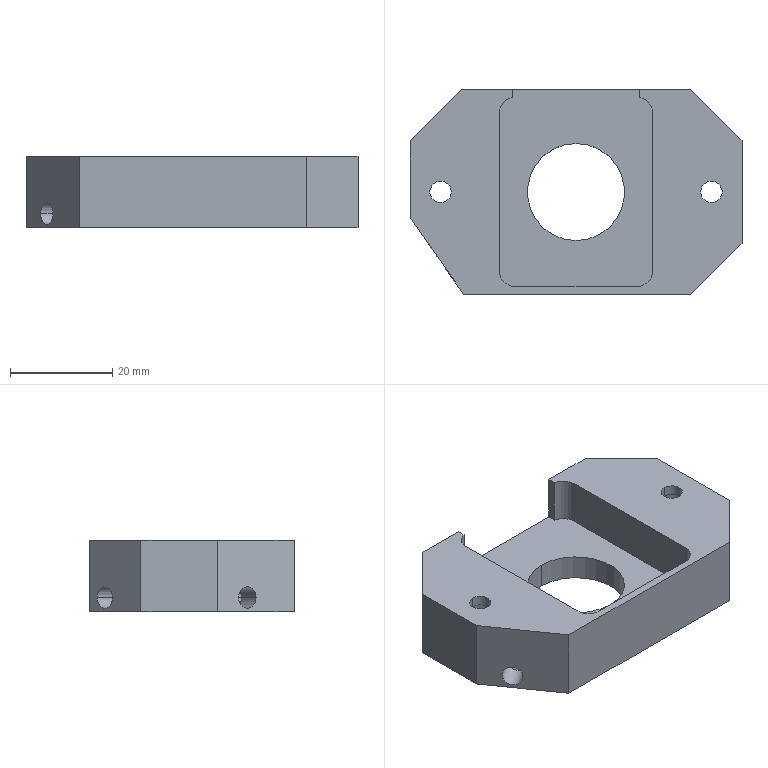NC program | NX | posted with a generic post | part box 65 x 40 x 14 mm
Whole program:
N10 G17 G21 G94 G90
(刀补10 , TOOL : 3.9XYD)
N12 T10 M6
N14 G54
N16 G17 G0 G90 X-26.5 Y0. S4000 M3
N18 G43 Z30. H10
N20 Z-11.365
N22 G42 G94 G1 X-26.516 Y0.099 F1000. D10
N24 G2 X-26.323 Y0.177 Z-11.5 R0.113
N26 X-26.323 Y0.177 Z-12.3 I-0.177 J-0.177
N28 X-26.323 Y0.177 Z-13.1 I-0.177 J-0.177
N30 X-26.323 Y0.177 Z-13.9 I-0.177 J-0.177
N32 X-26.25 Y0. Z-14. R0.25
N34 X-26.441 Y-0.081 Z-14.135 R0.113
N36 G40
N38 G1 X-26.5 Y0.
N40 G0 Z30.
N42 Z-11.342
N44 G42 G1 X-26.537 Y0.093
N46 G2 X-26.253 Y0.247 Z-11.5 R0.169
N48 X-26.253 Y0.247 Z-12.3 I-0.247 J-0.247
N50 X-26.253 Y0.247 Z-13.1 I-0.247 J-0.247
N52 X-26.253 Y0.247 Z-13.9 I-0.247 J-0.247
N54 X-26.15 Y0. Z-14. R0.35
N56 X-26.461 Y-0.092 Z-14.158 R0.169
N58 G40
N60 G1 X-26.5 Y0.
N62 G0 Z30.
N64 Z-11.33
N66 G42 G1 X-26.549 Y0.087
N68 G2 X-26.182 Y0.318 Z-11.5 R0.222
N70 X-26.182 Y0.318 Z-12.3 I-0.318 J-0.318
N72 X-26.182 Y0.318 Z-13.1 I-0.318 J-0.318
N74 X-26.182 Y0.318 Z-13.9 I-0.318 J-0.318
N76 X-26.05 Y0. Z-14. R0.45
N78 X-26.473 Y-0.096 Z-14.17 R0.222
N80 G40
N82 G1 X-26.5 Y0.
N84 G0 Z30.
N86 Z-11.324
N88 G42 G1 X-26.556 Y0.083
N90 G2 X-26.111 Y0.389 Z-11.5 R0.275
N92 X-26.111 Y0.389 Z-12.3 I-0.389 J-0.389
N94 X-26.111 Y0.389 Z-13.1 I-0.389 J-0.389
N96 X-26.111 Y0.389 Z-13.9 I-0.389 J-0.389
N98 X-25.95 Y0. Z-14. R0.55
N100 X-26.481 Y-0.098 Z-14.176 R0.275
N102 G40
N104 G1 X-26.5 Y0.
N106 G0 Z30.
N108 X26.5
N110 Z-11.365
N112 G42 G1 X26.484 Y0.099
N114 G2 X26.677 Y0.177 Z-11.5 R0.113
N116 X26.677 Y0.177 Z-12.3 I-0.177 J-0.177
N118 X26.677 Y0.177 Z-13.1 I-0.177 J-0.177
N120 X26.677 Y0.177 Z-13.9 I-0.177 J-0.177
N122 X26.75 Y0. Z-14. R0.25
N124 X26.559 Y-0.081 Z-14.135 R0.113
N126 G40
N128 G1 X26.5 Y0.
N130 G0 Z30.
N132 Z-11.342
N134 G42 G1 X26.463 Y0.093
N136 G2 X26.747 Y0.247 Z-11.5 R0.169
N138 X26.747 Y0.247 Z-12.3 I-0.247 J-0.247
N140 X26.747 Y0.247 Z-13.1 I-0.247 J-0.247
N142 X26.747 Y0.247 Z-13.9 I-0.247 J-0.247
N144 X26.85 Y0. Z-14. R0.35
N146 X26.539 Y-0.092 Z-14.158 R0.169
N148 G40
N150 G1 X26.5 Y0.
N152 G0 Z30.
N154 Z-11.33
N156 G42 G1 X26.451 Y0.087
N158 G2 X26.818 Y0.318 Z-11.5 R0.222
N160 X26.818 Y0.318 Z-12.3 I-0.318 J-0.318
N162 X26.818 Y0.318 Z-13.1 I-0.318 J-0.318
N164 X26.818 Y0.318 Z-13.9 I-0.318 J-0.318
N166 X26.95 Y0. Z-14. R0.45
N168 X26.527 Y-0.096 Z-14.17 R0.222
N170 G40
N172 G1 X26.5 Y0.
N174 G0 Z30.
N176 Z-11.324
N178 G42 G1 X26.444 Y0.083
N180 G2 X26.889 Y0.389 Z-11.5 R0.275
N182 X26.889 Y0.389 Z-12.3 I-0.389 J-0.389
N184 X26.889 Y0.389 Z-13.1 I-0.389 J-0.389
N186 X26.889 Y0.389 Z-13.9 I-0.389 J-0.389
N188 X27.05 Y0. Z-14. R0.55
N190 X26.519 Y-0.098 Z-14.176 R0.275
N192 G40
N194 G1 X26.5 Y0.
N196 G0 Z30.
N198 M5
(ZLEVEL_PROFILE_1_COPY , TOOL : D10JING)
N200 T14 M6
N202 G54
N204 G17 G0 G90 X-23.596 Y25.899 S6500 M3
N206 G43 Z30. H14
N208 Z-13.
N210 G94 G1 Z-14. F1000.
N212 X-23.366 Y25.5
N214 G3 X-22.5 Y25. R1.
N216 G1 X22.5
N218 G2 X26.036 Y23.536 R5.
N220 G1 X36.036 Y13.536
N222 G2 X37.5 Y10. R5.
N224 G1 Y-5.
N226 G2 X36.596 Y-7.868 R5.
N228 G1 X26.093 Y-22.868
N230 G2 X21.997 Y-25. R5.
N232 G1 X-22.5
N234 G2 X-26.036 Y-23.536 R5.
N236 G1 X-36.036 Y-13.536
N238 G2 X-37.5 Y-10. R5.
N240 G1 Y10.
N242 G2 X-36.036 Y13.536 R5.
N244 G1 X-26.036 Y23.536
N246 G2 X-22.5 Y25. R5.
N248 G3 X-21.634 Y25.5 R1.
N250 G1 X-21.345 Y26.
N252 Z-13.
N254 G0 Z30.
N256 M5
N258 M2